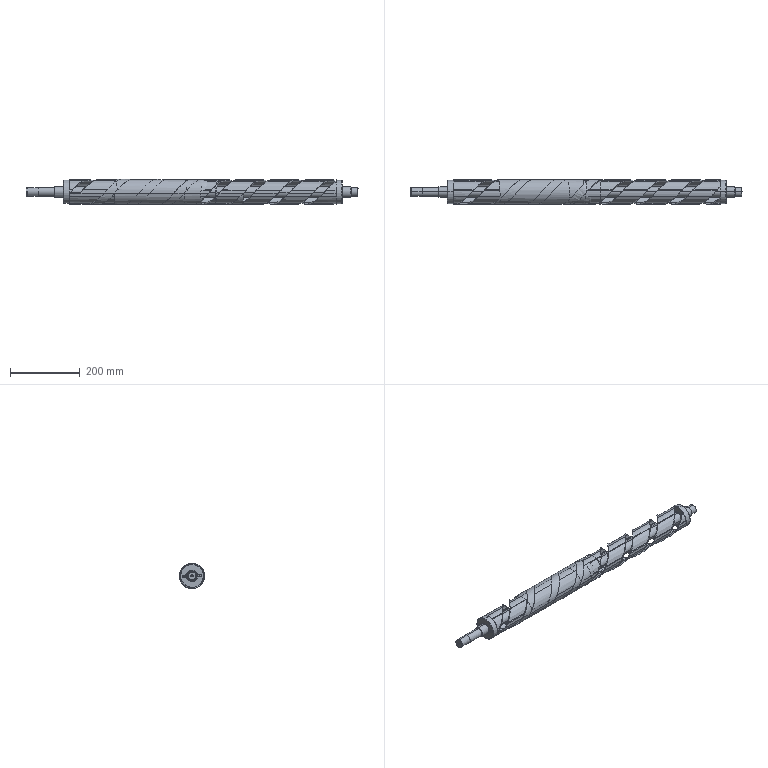Part | SolidWorks | features LayoutProfileFeature 1 | 5 solids | 271 faces | box 955.318 x 72.003 x 80.734 mm | volume 3264645 mm3 | cylinder 129 | plane 101 | cone 22 | spline 19 | commonest cylinder face diameters 70 x42 65 x34 72 x14 8 x7 7 x4 7.5 x4